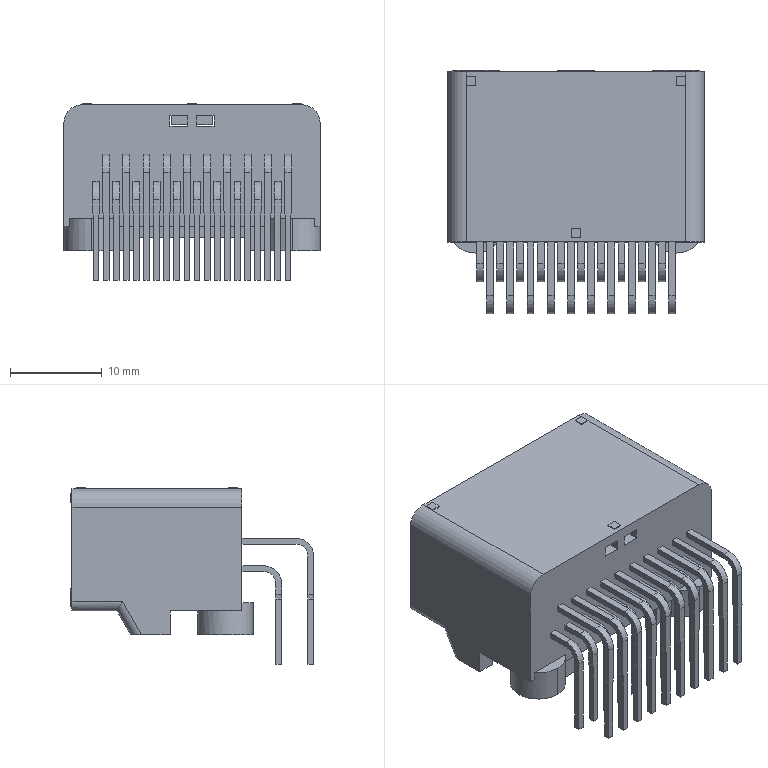Part | SolidWorks | 1 solid | 512 faces | box 27.9 x 26.52 x 19.2 mm | volume 3570 mm3 | plane 452 | cylinder 60 | commonest cylinder face diameters 2.64 x20 3.92 x20 6 x6 1 x4 2 x4 2.35 x4